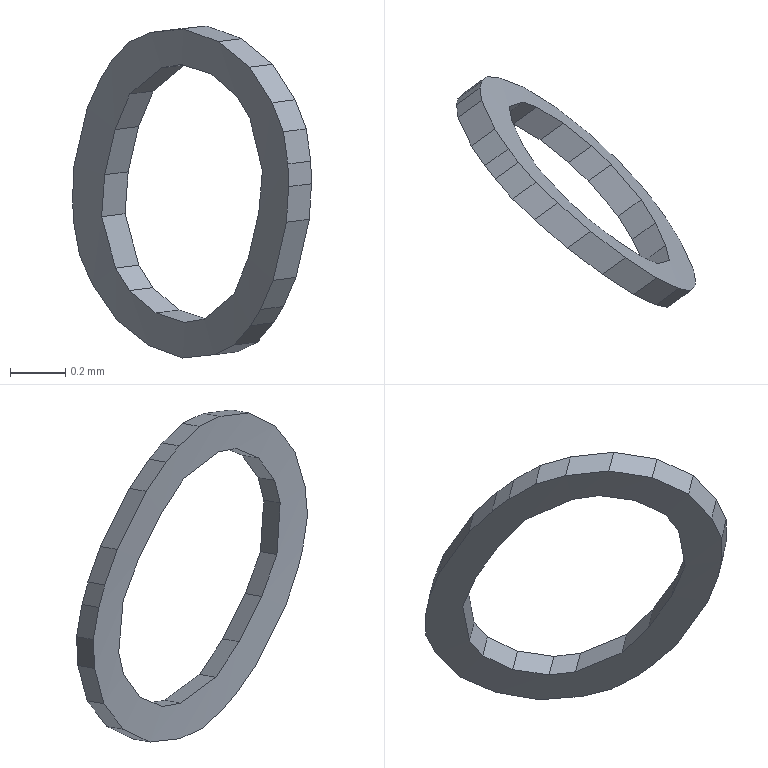Part | SolidWorks | features BaseBody 1 | 1 solid | 46 faces | box 0.8628 x 0.8341 x 1.199 mm | volume 0.04242 mm3 | plane 44 | cylinder 2 | commonest cylinder face diameters 16.8 x1 17 x1